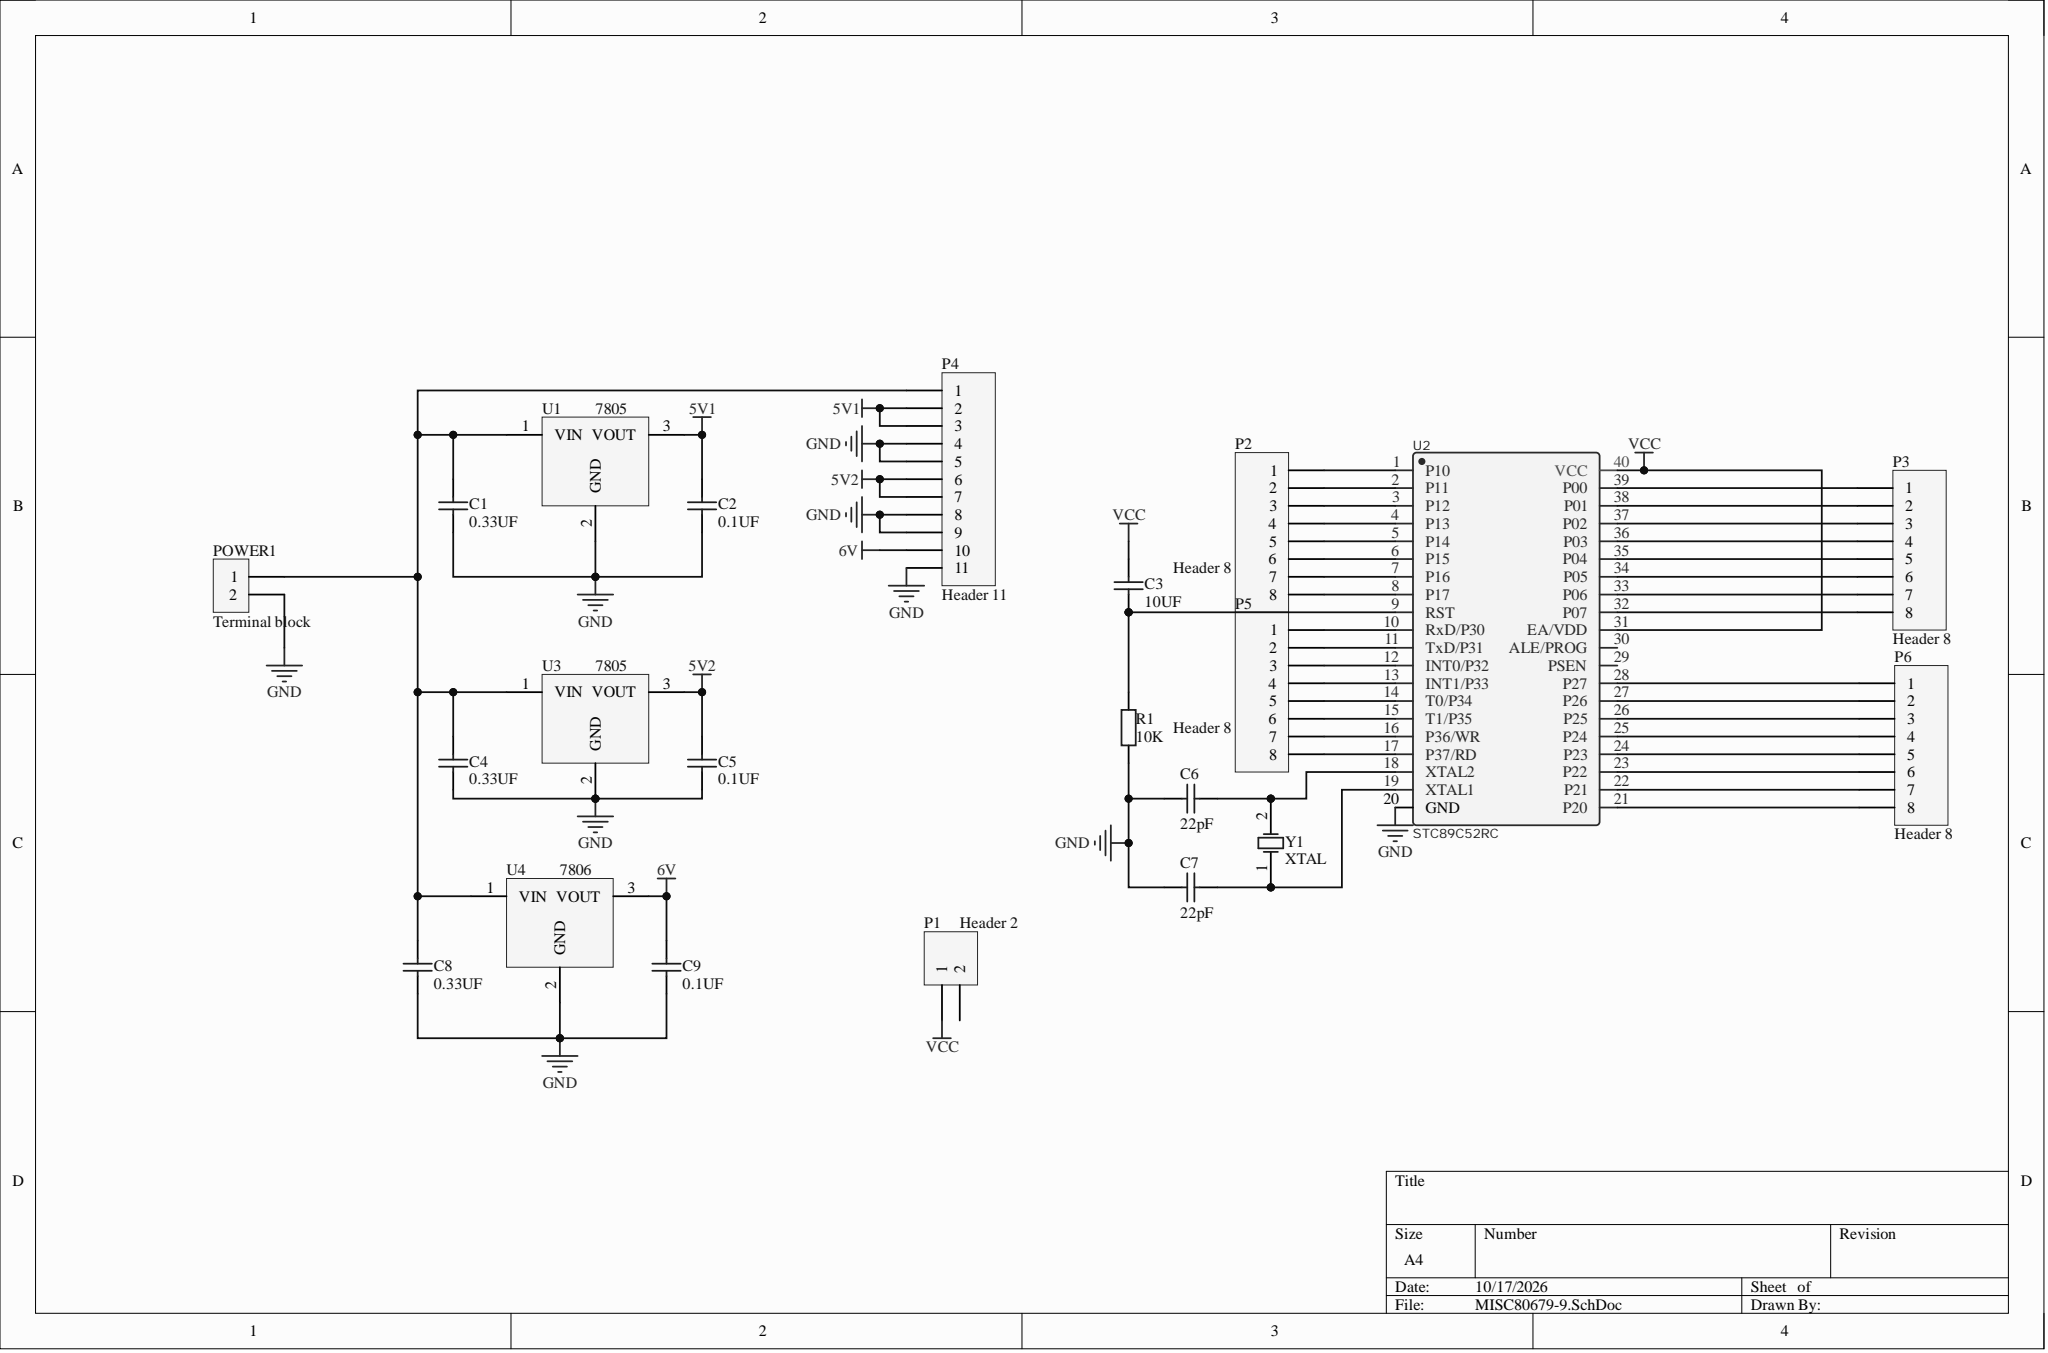Circuit board | Altium Designer | 22 parts | 41 nets
Bill of materials:
Comment,Description,Designator,Footprint,LibRef,Quantity
"0.33UF","Capacitor","C1, C4, C8","CC 1.8*3.6","Cap","3"
"0.1UF","Capacitor","C2, C5, C9","CC 1.8*3.6","Cap","3"
"10UF","Capacitor","C3","CAP 1.5*4*8","Cap","1"
"22pF","Capacitor","C6, C7","CC 1.8*3.6","Cap","2"
"Header 2","Header, 2-Pin","P1","HDR1X2","Header 2","1"
"Header 8","Header, 8-Pin","P2, P3, P5, P6","HDR1X8","Header 8","4"
"Header 11","Header, 11-Pin","P4","HDR1X11","Header 11","1"
"Terminal block","","POWER1","VH3.96-2A","VH2","1"
"10K","Resistor","R1","AXIAL-0.4","Res2","1"
"7805","","U1, U3","TO220A","LM7805","2"
"STC89C52RC","","U2","STC89C52RC","STC89C52RC","1"
"7806","","U4","TO220A","LM7805","1"
"XTAL","Crystal Oscillator","Y1","R38","XTAL","1"
Netlist (Protel format):
[
C1
CC 1.8*3.6
0.33UF



]
[
C2
CC 1.8*3.6
0.1UF



]
[
C3
CAP 1.5*4*8
10UF



]
[
C4
CC 1.8*3.6
0.33UF



]
[
C5
CC 1.8*3.6
0.1UF



]
[
C6
CC 1.8*3.6
22pF



]
[
C7
CC 1.8*3.6
22pF



]
[
C8
CC 1.8*3.6
0.33UF



]
[
C9
CC 1.8*3.6
0.1UF



]
[
P1
HDR1X2
Header 2



]
[
P2
HDR1X8
Header 8



]
[
P3
HDR1X8
Header 8



]
[
P4
HDR1X11
Header 11



]
[
P5
HDR1X8
Header 8



]
[
P6
HDR1X8
Header 8



]
[
POWER1
VH3.96-2A
Terminal block



]
[
R1
AXIAL-0.4
10K



]
[
U1
TO220A
7805



]
[
U2
STC89C52RC
STC89C52RC



]
[
U3
TO220A
7805



]
[
U4
TO220A
7806



]
[
Y1
R38
XTAL



]
(
VCC
C3-1
P1-1
U2-31
U2-40
)
(
NetP6_8
P6-8
U2-21
)
(
NetP6_7
P6-7
U2-22
)
(
NetP6_6
P6-6
U2-23
)
(
NetP6_5
P6-5
U2-24
)
(
NetP6_4
P6-4
U2-25
)
(
NetP6_3
P6-3
U2-26
)
(
NetP6_2
P6-2
U2-27
)
(
NetP6_1
P6-1
U2-28
)
(
NetP5_8
P5-8
U2-17
)
(
NetP5_7
P5-7
U2-16
)
(
NetP5_6
P5-6
U2-15
)
(
NetP5_5
P5-5
U2-14
)
(
NetP5_4
P5-4
U2-13
)
(
NetP5_3
P5-3
U2-12
)
(
NetP5_2
P5-2
U2-11
)
(
NetP5_1
P5-1
U2-10
)
(
NetP3_8
P3-8
U2-32
)
(
NetP3_7
P3-7
U2-33
)
(
NetP3_6
P3-6
U2-34
)
(
NetP3_5
P3-5
U2-35
)
(
NetP3_4
P3-4
U2-36
)
(
NetP3_3
P3-3
U2-37
)
(
NetP3_2
P3-2
U2-38
)
(
NetP3_1
P3-1
U2-39
)
(
NetP2_8
P2-8
U2-8
)
(
NetP2_7
P2-7
U2-7
)
(
NetP2_6
P2-6
U2-6
)
(
NetP2_5
P2-5
U2-5
)
(
NetP2_4
P2-4
U2-4
)
(
NetP2_3
P2-3
U2-3
)
(
NetP2_2
P2-2
U2-2
)
(
NetP2_1
P2-1
U2-1
)
(
NetC7_1
C7-1
U2-19
Y1-1
)
(
NetC6_1
C6-1
U2-18
Y1-2
)
(
NetC3_2
C3-2
R1-2
U2-9
)
(
NetC1_1
C1-1
C4-1
C8-1
P4-1
POWER1-1
U1-1
U3-1
U4-1
)
(
GND
C1-2
C2-2
C4-2
C5-2
C6-2
C7-2
C8-2
C9-2
P4-4
P4-5
P4-8
P4-9
P4-11
POWER1-2
R1-1
U1-2
U2-20
U3-2
U4-2
)
(
6V
C9-1
P4-10
U4-3
)
(
5V2
C5-1
P4-6
P4-7
U3-3
)
(
5V1
C2-1
P4-2
P4-3
U1-3
)